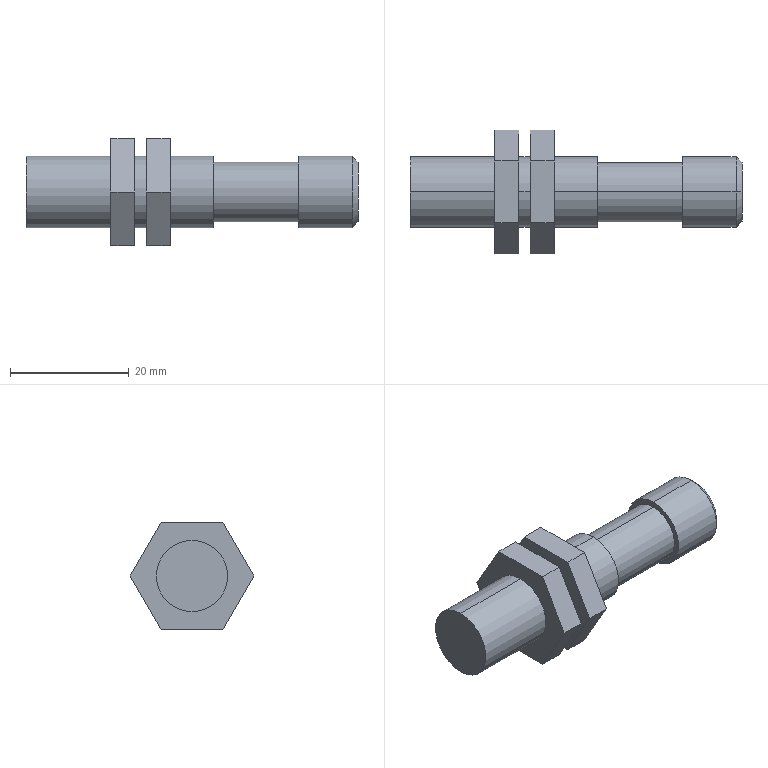Part | STEP file | Proximity switch | 1 solid | 32 faces | box 55.8 x 20.785 x 18 mm | volume 7139 mm3 | plane 20 | cylinder 10 | cone 2 | commonest cylinder face diameters 12 x8 10 x2